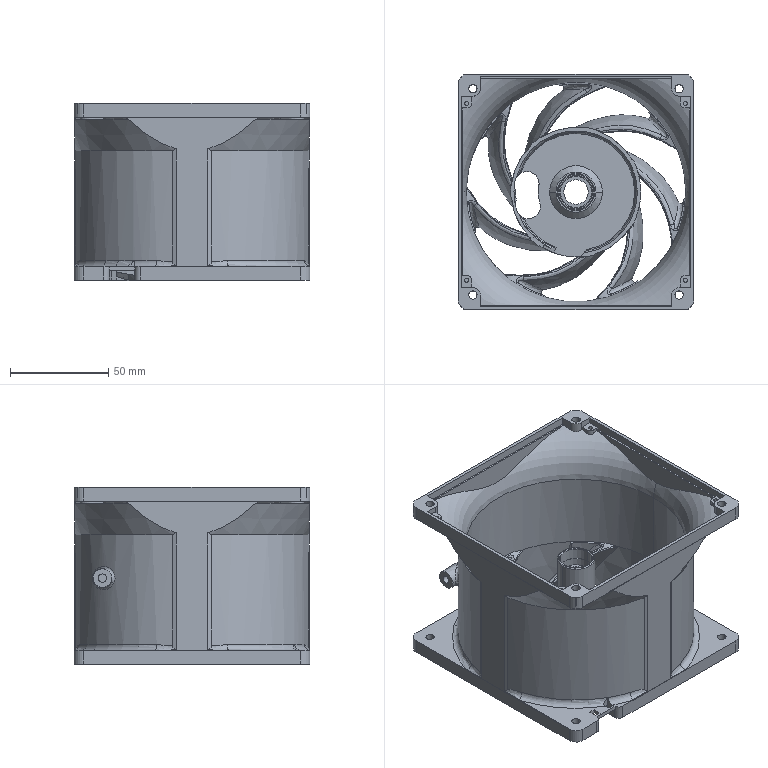NC program | NX | posted with a generic post | part box 120 x 120 x 90.2 mm
Lines 95260 to 96379 of 828686:
(等高精加工_COPY_COPY_COPY , TOOL : 4R0.5)
N190506 T08 M6
N190508 G54
N190510 G17 G0 G90 X-54.5 Y-42.233 S8000 M3
N190512 G43 Z140.7 H8
N190514 Z91.14
N190516 G94 G1 Z90.14 F1500.
N190518 X-54.89 Y-42.272
N190520 X-55.265 Y-42.386
N190522 X-55.611 Y-42.57
N190524 X-55.914 Y-42.819
N190526 X-56.163 Y-43.122
N190528 X-56.348 Y-43.468
N190530 X-56.462 Y-43.843
N190532 X-56.5 Y-44.233
N190534 Y-46.7
N190536 X-54.033
N190538 X-53.896 Z90.126
N190540 X-53.758 Z90.112
N190542 X-53.621 Z90.098
N190544 X-53.484 Z90.084
N190546 X-53.346 Z90.07
N190548 X-56.5
N190550 Y-43.547
N190552 Z90.
N190554 Y-46.7
N190556 X-53.346
N190558 Z89.93
N190560 X-56.5
N190562 Y-43.547
N190564 Z89.86
N190566 Y-46.7
N190568 X-53.346
N190570 Z89.79
N190572 X-56.5
N190574 Y-43.547
N190576 Z89.72
N190578 Y-46.7
N190580 X-53.346
N190582 X-53.347 Z89.65
N190584 X-56.5
N190586 Y-43.547
N190588 Z89.58
N190590 Y-46.7
N190592 X-53.347
N190594 Z89.51
N190596 X-56.5
N190598 Y-43.547
N190600 Z89.44
N190602 Y-46.7
N190604 X-53.347
N190606 Z89.37
N190608 X-56.5
N190610 Y-43.547
N190612 Z89.3
N190614 Y-46.7
N190616 X-53.347
N190618 Z89.23
N190620 X-56.5
N190622 Y-43.547
N190624 Z89.16
N190626 Y-46.7
N190628 X-53.347
N190630 Z89.09
N190632 X-56.5
N190634 Y-43.547
N190636 Z89.02
N190638 Y-46.7
N190640 X-53.347
N190642 Z88.95
N190644 X-56.5
N190646 Y-43.547
N190648 Z88.88
N190650 Y-46.7
N190652 X-53.347
N190654 Z88.81
N190656 X-56.5
N190658 Y-43.547
N190660 Z88.74
N190662 Y-46.7
N190664 X-53.347
N190666 Z88.67
N190668 X-56.5
N190670 Y-43.547
N190672 Z88.6
N190674 Y-46.7
N190676 X-53.347
N190678 Z88.53
N190680 X-56.5
N190682 Y-43.547
N190684 Z88.46
N190686 Y-46.7
N190688 X-53.347
N190690 Z88.39
N190692 X-56.5
N190694 Y-43.547
N190696 Z88.32
N190698 Y-46.7
N190700 X-53.347
N190702 Z88.25
N190704 X-56.5
N190706 Y-43.547
N190708 Z88.18
N190710 Y-46.7
N190712 X-53.347
N190714 Z88.11
N190716 X-56.5
N190718 Y-43.547
N190720 Z88.04
N190722 Y-46.7
N190724 X-53.347
N190726 Z87.97
N190728 X-56.5
N190730 Y-43.547
N190732 Z87.9
N190734 Y-46.7
N190736 X-53.347
N190738 Z87.83
N190740 X-56.5
N190742 Y-43.547
N190744 Z87.76
N190746 Y-46.7
N190748 X-53.347
N190750 Z87.69
N190752 X-56.5
N190754 Y-43.547
N190756 Z87.62
N190758 Y-46.7
N190760 X-53.347
N190762 Z87.55
N190764 X-56.5
N190766 Y-43.547
N190768 Z87.48
N190770 Y-46.7
N190772 X-53.347
N190774 Z87.41
N190776 X-56.5
N190778 Y-43.547
N190780 Z87.34
N190782 Y-46.7
N190784 X-53.347
N190786 Z87.27
N190788 X-56.5
N190790 Y-43.547
N190792 Z87.2
N190794 Y-46.7
N190796 X-53.347
N190798 Z87.185
N190800 X-56.5
N190802 Y-43.547
N190804 Z87.161
N190806 Y-46.7
N190808 X-53.347
N190810 Z87.128
N190812 X-56.5
N190814 Y-43.547
N190816 Z87.087
N190818 Y-46.7
N190820 X-53.347
N190822 Z87.038
N190824 X-56.5
N190826 Y-43.547
N190828 Z86.982
N190830 Y-46.7
N190832 X-53.347
N190834 Z86.922
N190836 X-56.5
N190838 Y-43.547
N190840 Z86.857
N190842 Y-46.7
N190844 X-53.347
N190846 Z86.789
N190848 X-56.5
N190850 Y-43.547
N190852 Z86.719
N190854 Y-46.7
N190856 X-53.347
N190858 Z86.649
N190860 X-56.5
N190862 Y-43.547
N190864 Z86.579
N190866 Y-46.7
N190868 X-53.347
N190870 Z86.509
N190872 X-56.5
N190874 Y-43.547
N190876 Z86.439
N190878 Y-46.7
N190880 X-53.347
N190882 Z86.379
N190884 X-56.5
N190886 Y-43.547
N190888 X-56.462 Y-43.157
N190890 X-56.348 Y-42.782
N190892 X-56.163 Y-42.436
N190894 X-55.914 Y-42.133
N190896 X-55.611 Y-41.884
N190898 X-55.265 Y-41.699
N190900 X-54.89 Y-41.585
N190902 X-54.5 Y-41.547
N190904 Z87.379
N190906 G0 Z140.7
N190908 X-44.7 Y-52.032
N190910 Z91.14
N190912 G1 Z90.14
N190914 X-45.09 Y-52.071
N190916 X-45.466 Y-52.185
N190918 X-45.811 Y-52.369
N190920 X-46.114 Y-52.618
N190922 X-46.363 Y-52.921
N190924 X-46.548 Y-53.267
N190926 X-46.662 Y-53.642
N190928 X-46.7 Y-54.032
N190930 Y-56.5
N190932 X-44.232
N190934 X-44.095 Z90.126
N190936 X-43.957 Z90.112
N190938 X-43.819 Z90.098
N190940 X-43.682 Z90.084
N190942 X-43.544 Z90.07
N190944 X-46.7
N190946 Y-53.345
N190948 Z90.
N190950 Y-56.5
N190952 X-43.544
N190954 Z89.93
N190956 X-46.7
N190958 Y-53.345
N190960 Z89.86
N190962 Y-56.5
N190964 X-43.544
N190966 Z89.79
N190968 X-46.7
N190970 Y-53.345
N190972 Y-53.344 Z89.72
N190974 Y-56.5
N190976 X-43.544
N190978 X-43.546 Z89.65
N190980 X-46.7
N190982 Y-53.346
N190984 Y-53.347 Z89.58
N190986 Y-56.5
N190988 X-43.547
N190990 Z89.51
N190992 X-46.7
N190994 Y-53.347
N190996 Z89.44
N190998 Y-56.5
N191000 X-43.547
N191002 Z89.37
N191004 X-46.7
N191006 Y-53.347
N191008 Z89.3
N191010 Y-56.5
N191012 X-43.547
N191014 Z89.23
N191016 X-46.7
N191018 Y-53.347
N191020 Z89.16
N191022 Y-56.5
N191024 X-43.547
N191026 Z89.09
N191028 X-46.7
N191030 Y-53.347
N191032 Z89.02
N191034 Y-56.5
N191036 X-43.547
N191038 Z88.95
N191040 X-46.7
N191042 Y-53.347
N191044 Z88.88
N191046 Y-56.5
N191048 X-43.547
N191050 Z88.81
N191052 X-46.7
N191054 Y-53.347
N191056 Z88.74
N191058 Y-56.5
N191060 X-43.547
N191062 Z88.67
N191064 X-46.7
N191066 Y-53.347
N191068 Z88.6
N191070 Y-56.5
N191072 X-43.547
N191074 Z88.53
N191076 X-46.7
N191078 Y-53.347
N191080 Z88.46
N191082 Y-56.5
N191084 X-43.547
N191086 Z88.39
N191088 X-46.7
N191090 Y-53.347
N191092 Z88.32
N191094 Y-56.5
N191096 X-43.547
N191098 Z88.25
N191100 X-46.7
N191102 Y-53.347
N191104 Z88.18
N191106 Y-56.5
N191108 X-43.547
N191110 Z88.11
N191112 X-46.7
N191114 Y-53.347
N191116 Z88.04
N191118 Y-56.5
N191120 X-43.547
N191122 Z87.97
N191124 X-46.7
N191126 Y-53.347
N191128 Z87.9
N191130 Y-56.5
N191132 X-43.547
N191134 Z87.83
N191136 X-46.7
N191138 Y-53.347
N191140 Z87.76
N191142 Y-56.5
N191144 X-43.547
N191146 Z87.69
N191148 X-46.7
N191150 Y-53.347
N191152 Z87.62
N191154 Y-56.5
N191156 X-43.547
N191158 Z87.55
N191160 X-46.7
N191162 Y-53.347
N191164 Z87.48
N191166 Y-56.5
N191168 X-43.547
N191170 Z87.41
N191172 X-46.7
N191174 Y-53.347
N191176 Z87.34
N191178 Y-56.5
N191180 X-43.547
N191182 Z87.27
N191184 X-46.7
N191186 Y-53.347
N191188 Z87.2
N191190 Y-56.5
N191192 X-43.547
N191194 X-43.157 Y-56.462
N191196 X-42.782 Y-56.348
N191198 X-42.436 Y-56.163
N191200 X-42.133 Y-55.914
N191202 X-41.884 Y-55.611
N191204 X-41.699 Y-55.265
N191206 X-41.585 Y-54.89
N191208 X-41.547 Y-54.5
N191210 Z88.2
N191212 G0 Z93.7
N191214 X-36.235
N191216 Z88.185
N191218 G1 Z87.185
N191220 X-36.273 Y-54.89
N191222 X-36.387 Y-55.265
N191224 X-36.572 Y-55.611
N191226 X-36.821 Y-55.914
N191228 X-37.124 Y-56.163
N191230 X-37.47 Y-56.348
N191232 X-37.845 Y-56.462
N191234 X-38.235 Y-56.5
N191236 X-41.078
N191238 Y-55.5
N191240 X-41.102 Y-55.061
N191242 X-41.172 Y-54.628
N191244 X-41.115 Y-54.701 Z87.173
N191246 X-41.069 Y-54.776 Z87.161
N191248 X-41.022 Y-55.137
N191250 X-41.006 Y-55.5
N191252 Y-56.5
N191254 X-38.235
N191256 Z87.128
N191258 X-40.941
N191260 Y-55.5
N191262 X-40.973 Y-54.982
N191264 X-41.067 Y-54.471
N191266 X-40.986 Y-54.562 Z87.087
N191268 X-40.909 Y-55.028
N191270 X-40.883 Y-55.5
N191272 Y-56.5
N191274 X-38.056
N191276 X-37.967 Z87.038
N191278 X-40.831
N191280 Y-55.5
N191282 X-40.854 Y-55.059
N191284 X-40.92 Y-54.623
N191286 X-41.03 Y-54.196
N191288 X-40.981 Y-54.279 Z87.01
N191290 X-40.936 Y-54.365 Z86.982
N191292 X-40.825 Y-54.927
N191294 X-40.787 Y-55.5
N191296 Y-56.5
N191298 X-37.967
N191300 X-37.908 Z86.922
N191302 X-40.752
N191304 Y-55.5
N191306 X-40.786 Y-54.95
N191308 X-40.888 Y-54.408
N191310 X-40.853 Y-54.438 Z86.857
N191312 X-40.757 Y-54.965
N191314 X-40.725 Y-55.5
N191316 Y-56.5
N191318 X-37.867
N191320 X-37.839 Z86.789
N191322 X-40.708
N191324 Y-55.5
N191326 X-40.731 Y-55.045
N191328 X-40.8 Y-54.594
N191330 X-40.792 Y-54.598 Z86.719
N191332 X-40.723 Y-55.047
N191334 X-40.7 Y-55.5
N191336 Y-56.5
N191338 X-37.824
N191340 X-37.819 Z86.649
N191342 X-40.7
N191344 Y-55.5
N191346 X-40.726 Y-55.019
N191348 X-40.803 Y-54.543
N191350 X-40.93 Y-54.079
N191352 Z86.579
N191354 X-40.803 Y-54.543
N191356 X-40.726 Y-55.019
N191358 X-40.7 Y-55.5
N191360 Y-56.5
N191362 X-37.819
N191364 Z86.509
N191366 X-40.7
N191368 Y-55.5
N191370 X-40.726 Y-55.019
N191372 X-40.803 Y-54.543
N191374 X-40.93 Y-54.079
N191376 Z86.439
N191378 X-40.803 Y-54.543
N191380 X-40.726 Y-55.019
N191382 X-40.7 Y-55.5
N191384 Y-56.5
N191386 X-37.819
N191388 Z86.379
N191390 X-40.7
N191392 Y-55.5
N191394 X-40.726 Y-55.019
N191396 X-40.803 Y-54.543
N191398 X-40.93 Y-54.079
N191400 X-41.017 Y-53.696
N191402 X-41.028 Y-53.304
N191404 X-40.962 Y-52.918
N191406 X-40.821 Y-52.552
N191408 X-40.612 Y-52.22
N191410 X-40.343 Y-51.935
N191412 X-40.023 Y-51.709
N191414 X-39.664 Y-51.549
N191416 Z87.379
N191418 G0 Z140.7
N191420 X-46.824 Y-46.914
N191422 Z88.185
N191424 G1 Z87.185
N191426 X-47.141 Y-47.146
N191428 X-47.406 Y-47.434
N191430 X-47.61 Y-47.769
N191432 X-47.745 Y-48.137
N191434 X-47.805 Y-48.525
N191436 X-47.789 Y-48.916
N191438 X-47.696 Y-49.297
N191440 X-47.531 Y-49.653
N191442 X-47.244 Y-50.203
N191444 X-47.015 Y-50.781
N191446 X-46.847 Y-51.378
N191448 X-45.519
N191450 X-45.628 Y-51.338 Z87.173
N191452 X-45.736 Y-51.306 Z87.161
N191454 X-46.864
N191456 X-47.031 Y-50.734
N191458 X-47.254 Y-50.181
N191460 X-47.531 Y-49.653
N191462 Z87.128
N191464 X-47.264 Y-50.161
N191466 X-47.046 Y-50.692
N191468 X-46.88 Y-51.241
N191470 X-45.342
N191472 X-45.41 Y-51.21 Z87.107
N191474 X-45.478 Y-51.183 Z87.087
N191476 X-46.895
N191478 X-47.075 Y-50.612
N191480 X-47.311 Y-50.061
N191482 X-47.601 Y-49.537
N191484 X-47.637 Y-49.48 Z87.038
N191486 X-47.339 Y-50.005
N191488 X-47.096 Y-50.557
N191490 X-46.909 Y-51.131
N191492 X-45.2
N191494 X-45.101 Y-51.132
N191496 X-45.002 Y-51.136
N191498 X-45.121 Y-51.108 Z87.01
N191500 X-45.24 Y-51.087 Z86.982
N191502 X-46.921
N191504 X-47.107 Y-50.529
N191506 X-47.346 Y-49.992
N191508 X-47.637 Y-49.48
N191510 X-47.662 Y-49.442 Z86.922
N191512 X-47.365 Y-49.954
N191514 X-47.121 Y-50.492
N191516 X-46.931 Y-51.052
N191518 X-45.308
N191520 X-45.353 Y-51.025 Z86.857
N191522 X-46.938
N191524 X-47.132 Y-50.465
N191526 X-47.379 Y-49.927
N191528 X-47.679 Y-49.416
N191530 X-47.69 Y-49.398 Z86.789
N191532 X-47.388 Y-49.909
N191534 X-47.139 Y-50.448
N191536 X-46.944 Y-51.008
N191538 X-45.563
N191540 X-45.57 Y-51. Z86.719
N191542 X-46.946
N191544 X-47.142 Y-50.439
N191546 X-47.393 Y-49.9
N191548 X-47.697 Y-49.388
N191550 X-47.699 Y-49.385 Z86.649
N191552 X-47.395 Y-49.898
N191554 X-47.143 Y-50.438
N191556 X-46.946 Y-51.
N191558 X-45.2
N191560 X-45.044 Y-51.003
N191562 X-44.888 Y-51.011
N191564 Z86.579
N191566 X-45.044 Y-51.003
N191568 X-45.2 Y-51.
N191570 X-46.946
N191572 X-47.143 Y-50.438
N191574 X-47.395 Y-49.898
N191576 X-47.699 Y-49.385
N191578 Z86.509
N191580 X-47.395 Y-49.898
N191582 X-47.143 Y-50.438
N191584 X-46.946 Y-51.
N191586 X-45.2
N191588 X-45.044 Y-51.003
N191590 X-44.888 Y-51.011
N191592 Z86.439
N191594 X-45.044 Y-51.003
N191596 X-45.2 Y-51.
N191598 X-46.946
N191600 X-47.143 Y-50.438
N191602 X-47.395 Y-49.898
N191604 X-47.699 Y-49.385
N191606 Z86.379
N191608 X-47.395 Y-49.898
N191610 X-47.143 Y-50.438
N191612 X-46.946 Y-51.
N191614 X-45.2
N191616 X-45.044 Y-51.003
N191618 X-44.888 Y-51.011
N191620 Z86.32
N191622 X-45.044 Y-51.003
N191624 X-45.2 Y-51.
N191626 X-46.946
N191628 X-47.143 Y-50.438
N191630 X-47.395 Y-49.898
N191632 X-47.699 Y-49.385
N191634 Z86.26
N191636 X-47.395 Y-49.898
N191638 X-47.143 Y-50.438
N191640 X-46.946 Y-51.
N191642 X-45.2
N191644 X-45.044 Y-51.003
N191646 X-44.888 Y-51.011
N191648 Z86.2
N191650 X-45.044 Y-51.003
N191652 X-45.2 Y-51.
N191654 X-46.946
N191656 X-47.143 Y-50.438
N191658 X-47.395 Y-49.898
N191660 X-47.699 Y-49.385
N191662 Z86.185
N191664 X-47.395 Y-49.898
N191666 X-47.143 Y-50.438
N191668 X-46.946 Y-51.
N191670 X-45.2
N191672 X-45.044 Y-51.003
N191674 X-44.888 Y-51.011
N191676 Z86.161
N191678 X-45.044 Y-51.003
N191680 X-45.2 Y-51.
N191682 X-46.946
N191684 X-47.143 Y-50.438
N191686 X-47.395 Y-49.898
N191688 X-47.699 Y-49.385
N191690 Z86.128
N191692 X-47.395 Y-49.898
N191694 X-47.143 Y-50.438
N191696 X-46.946 Y-51.
N191698 X-45.2
N191700 X-45.044 Y-51.003
N191702 X-44.888 Y-51.011
N191704 Z86.087
N191706 X-45.044 Y-51.003
N191708 X-45.2 Y-51.
N191710 X-46.946
N191712 X-47.143 Y-50.438
N191714 X-47.395 Y-49.898
N191716 X-47.699 Y-49.385
N191718 Z86.038
N191720 X-47.395 Y-49.898
N191722 X-47.143 Y-50.438
N191724 X-46.946 Y-51.
N191726 X-45.2
N191728 X-45.044 Y-51.003
N191730 X-44.888 Y-51.011
N191732 Z85.983
N191734 X-45.044 Y-51.003
N191736 X-45.2 Y-51.
N191738 X-46.946
N191740 X-47.143 Y-50.438
N191742 X-47.395 Y-49.898
N191744 X-47.699 Y-49.385
N191746 Z85.976
N191748 X-47.395 Y-49.898
N191750 X-47.143 Y-50.438
N191752 X-46.946 Y-51.
N191754 X-45.2
N191756 X-45.044 Y-51.003
N191758 X-44.888 Y-51.011
N191760 Z85.969
N191762 X-45.044 Y-51.003
N191764 X-45.2 Y-51.
N191766 X-46.946
N191768 X-47.143 Y-50.438
N191770 X-47.395 Y-49.898
N191772 X-47.699 Y-49.385
N191774 Z85.963
N191776 X-47.395 Y-49.898
N191778 X-47.143 Y-50.438
N191780 X-46.946 Y-51.
N191782 X-45.2
N191784 X-45.044 Y-51.003
N191786 X-44.888 Y-51.011
N191788 Z85.956
N191790 X-45.044 Y-51.003
N191792 X-45.2 Y-51.
N191794 X-46.946
N191796 X-47.143 Y-50.438
N191798 X-47.395 Y-49.898
N191800 X-47.699 Y-49.385
N191802 Z85.949
N191804 X-47.395 Y-49.898
N191806 X-47.143 Y-50.438
N191808 X-46.946 Y-51.
N191810 X-45.2
N191812 X-45.044 Y-51.003
N191814 X-44.888 Y-51.011
N191816 Z85.942
N191818 X-45.044 Y-51.003
N191820 X-45.2 Y-51.
N191822 X-46.946
N191824 X-47.143 Y-50.438
N191826 X-47.395 Y-49.898
N191828 X-47.699 Y-49.385
N191830 Z85.935
N191832 X-47.395 Y-49.898
N191834 X-47.143 Y-50.438
N191836 X-46.946 Y-51.
N191838 X-45.2
N191840 X-45.044 Y-51.003
N191842 X-44.888 Y-51.011
N191844 Z85.927
N191846 X-45.044 Y-51.003
N191848 X-45.2 Y-51.
N191850 X-46.946
N191852 X-47.143 Y-50.438
N191854 X-47.395 Y-49.898
N191856 X-47.699 Y-49.385
N191858 Z85.919
N191860 X-47.395 Y-49.898
N191862 X-47.143 Y-50.438
N191864 X-46.946 Y-51.
N191866 X-45.2
N191868 X-45.044 Y-51.003
N191870 X-44.888 Y-51.011
N191872 Z85.911
N191874 X-45.044 Y-51.003
N191876 X-45.2 Y-51.
N191878 X-46.946
N191880 X-47.143 Y-50.438
N191882 X-47.395 Y-49.898
N191884 X-47.699 Y-49.385
N191886 Z85.903
N191888 X-47.395 Y-49.898
N191890 X-47.143 Y-50.438
N191892 X-46.946 Y-51.
N191894 X-45.2
N191896 X-45.044 Y-51.003
N191898 X-44.888 Y-51.011
N191900 Z85.894
N191902 X-45.044 Y-51.003
N191904 X-45.2 Y-51.
N191906 X-46.946
N191908 X-47.143 Y-50.438
N191910 X-47.395 Y-49.898
N191912 X-47.699 Y-49.385
N191914 Z85.886
N191916 X-47.395 Y-49.898
N191918 X-47.143 Y-50.438
N191920 X-46.946 Y-51.
N191922 X-45.2
N191924 X-45.044 Y-51.003
N191926 X-44.888 Y-51.011
N191928 Z85.877
N191930 X-45.044 Y-51.003
N191932 X-45.2 Y-51.
N191934 X-46.946
N191936 X-47.143 Y-50.438
N191938 X-47.395 Y-49.898
N191940 X-47.699 Y-49.385
N191942 Z85.867
N191944 X-47.395 Y-49.898
N191946 X-47.143 Y-50.438
N191948 X-46.946 Y-51.
N191950 X-45.2
N191952 X-45.044 Y-51.003
N191954 X-44.888 Y-51.011
N191956 Z85.858
N191958 X-45.044 Y-51.003
N191960 X-45.2 Y-51.
N191962 X-46.946
N191964 X-47.143 Y-50.438
N191966 X-47.395 Y-49.898
N191968 X-47.699 Y-49.385
N191970 Z85.848
N191972 X-47.395 Y-49.898
N191974 X-47.143 Y-50.438
N191976 X-46.946 Y-51.
N191978 X-45.2
N191980 X-45.044 Y-51.003
N191982 X-44.888 Y-51.011
N191984 Z85.838
N191986 X-45.044 Y-51.003
N191988 X-45.2 Y-51.
N191990 X-46.946
N191992 X-47.143 Y-50.438
N191994 X-47.395 Y-49.898
N191996 X-47.699 Y-49.385
N191998 Z85.828
N192000 X-47.395 Y-49.898
N192002 X-47.143 Y-50.438
N192004 X-46.946 Y-51.
N192006 X-45.2
N192008 X-45.044 Y-51.003
N192010 X-44.888 Y-51.011
N192012 Z85.817
N192014 X-45.044 Y-51.003
N192016 X-45.2 Y-51.
N192018 X-46.946
N192020 X-47.143 Y-50.438
N192022 X-47.395 Y-49.898
N192024 X-47.699 Y-49.385
N192026 Z85.807
N192028 X-47.395 Y-49.898
N192030 X-47.143 Y-50.438
N192032 X-46.946 Y-51.
N192034 X-45.2
N192036 X-45.044 Y-51.003
N192038 X-44.888 Y-51.011
N192040 Z85.796
N192042 X-45.044 Y-51.003
N192044 X-45.2 Y-51.
N192046 X-46.946
N192048 X-47.143 Y-50.438
N192050 X-47.395 Y-49.898
N192052 X-47.699 Y-49.385
N192054 Z85.785
N192056 X-47.395 Y-49.898
N192058 X-47.143 Y-50.438
N192060 X-46.946 Y-51.
N192062 X-45.2
N192064 X-45.044 Y-51.003
N192066 X-44.888 Y-51.011
N192068 Z85.773
N192070 X-45.044 Y-51.003
N192072 X-45.2 Y-51.
N192074 X-46.946
N192076 X-47.143 Y-50.438
N192078 X-47.395 Y-49.898
N192080 X-47.699 Y-49.385
N192082 Z85.761
N192084 X-47.395 Y-49.898
N192086 X-47.143 Y-50.438
N192088 X-46.946 Y-51.
N192090 X-45.2
N192092 X-45.044 Y-51.003
N192094 X-44.888 Y-51.011
N192096 Z85.75
N192098 X-45.044 Y-51.003
N192100 X-45.2 Y-51.
N192102 X-46.946
N192104 X-47.143 Y-50.438
N192106 X-47.395 Y-49.898
N192108 X-47.699 Y-49.385
N192110 Z85.737
N192112 X-47.395 Y-49.898
N192114 X-47.143 Y-50.438
N192116 X-46.946 Y-51.
N192118 X-45.2
N192120 X-45.044 Y-51.003
N192122 X-44.888 Y-51.011
N192124 Z85.725
N192126 X-45.044 Y-51.003
N192128 X-45.2 Y-51.
N192130 X-46.946
N192132 X-47.143 Y-50.438
N192134 X-47.395 Y-49.898
N192136 X-47.699 Y-49.385
N192138 Z85.713
N192140 X-47.395 Y-49.898
N192142 X-47.143 Y-50.438
N192144 X-46.946 Y-51.
N192146 X-45.2
N192148 X-45.044 Y-51.003
N192150 X-44.888 Y-51.011
N192152 Z85.7
N192154 X-45.044 Y-51.003
N192156 X-45.2 Y-51.
N192158 X-46.946
N192160 X-47.143 Y-50.438
N192162 X-47.395 Y-49.898
N192164 X-47.699 Y-49.385
N192166 Z85.687
N192168 X-47.395 Y-49.898
N192170 X-47.143 Y-50.438
N192172 X-46.946 Y-51.
N192174 X-45.2
N192176 X-45.044 Y-51.003
N192178 X-44.888 Y-51.011
N192180 Z85.673
N192182 X-45.044 Y-51.003
N192184 X-45.2 Y-51.
N192186 X-46.946
N192188 X-47.143 Y-50.438
N192190 X-47.395 Y-49.898
N192192 X-47.699 Y-49.385
N192194 Z85.66
N192196 X-47.395 Y-49.898
N192198 X-47.143 Y-50.438
N192200 X-46.946 Y-51.
N192202 X-45.2
N192204 X-45.044 Y-51.003
N192206 X-44.888 Y-51.011
N192208 Z85.646
N192210 X-45.044 Y-51.003
N192212 X-45.2 Y-51.
N192214 X-46.946
N192216 X-47.143 Y-50.438
N192218 X-47.395 Y-49.898
N192220 X-47.699 Y-49.385
N192222 Z85.632
N192224 X-47.395 Y-49.898
N192226 X-47.143 Y-50.438
N192228 X-46.946 Y-51.
N192230 X-45.2
N192232 X-45.044 Y-51.003
N192234 X-44.888 Y-51.011
N192236 Z85.618
N192238 X-45.044 Y-51.003
N192240 X-45.2 Y-51.
N192242 X-46.946
N192244 X-47.143 Y-50.438
N192246 X-47.395 Y-49.898
N192248 X-47.699 Y-49.385
N192250 Z85.603
N192252 X-47.395 Y-49.898
N192254 X-47.143 Y-50.438
N192256 X-46.946 Y-51.
N192258 X-45.2
N192260 X-45.044 Y-51.003
N192262 X-44.888 Y-51.011
N192264 Z85.589
N192266 X-45.044 Y-51.003
N192268 X-45.2 Y-51.
N192270 X-46.946
N192272 X-47.143 Y-50.438
N192274 X-47.395 Y-49.898
N192276 X-47.699 Y-49.385
N192278 Z85.574
N192280 X-47.395 Y-49.898
N192282 X-47.143 Y-50.438
N192284 X-46.946 Y-51.
N192286 X-45.2
N192288 X-45.044 Y-51.003
N192290 X-44.888 Y-51.011
N192292 Z85.559
N192294 X-45.044 Y-51.003
N192296 X-45.2 Y-51.
N192298 X-46.946
N192300 X-47.143 Y-50.438
N192302 X-47.395 Y-49.898
N192304 X-47.699 Y-49.385
N192306 Z85.543
N192308 X-47.395 Y-49.898
N192310 X-47.143 Y-50.438
N192312 X-46.946 Y-51.
N192314 X-45.2
N192316 X-45.044 Y-51.003
N192318 X-44.888 Y-51.011
N192320 Z85.528
N192322 X-45.044 Y-51.003
N192324 X-45.2 Y-51.
N192326 X-46.946
N192328 X-47.143 Y-50.438
N192330 X-47.395 Y-49.898
N192332 X-47.699 Y-49.385
N192334 Z85.512
N192336 X-47.395 Y-49.898
N192338 X-47.143 Y-50.438
N192340 X-46.946 Y-51.
N192342 X-45.2
N192344 X-45.044 Y-51.003
N192346 X-44.888 Y-51.011
N192348 Z85.496
N192350 X-45.044 Y-51.003
N192352 X-45.2 Y-51.
N192354 X-46.946
N192356 X-47.143 Y-50.438
N192358 X-47.395 Y-49.898
N192360 X-47.699 Y-49.385
N192362 X-47.714 Y-49.363 Z85.479
N192364 X-47.403 Y-49.882
N192366 X-47.146 Y-50.429
N192368 X-46.946 Y-51.
N192370 X-45.2
N192372 X-45.044 Y-51.003
N192374 X-44.888 Y-51.011
N192376 X-44.88 Z85.463
N192378 X-45.04 Y-51.003
N192380 X-45.2 Y-51.
N192382 X-46.946
N192384 X-47.159 Y-50.399
N192386 X-47.434 Y-49.824
N192388 X-47.769 Y-49.281
N192390 X-47.699 Y-49.385 Z85.446
N192392 X-47.395 Y-49.898
N192394 X-47.143 Y-50.438
N192396 X-46.946 Y-51.
N192398 X-45.2
N192400 X-45.044 Y-51.003
N192402 X-44.888 Y-51.011
N192404 Z85.429
N192406 X-45.044 Y-51.003
N192408 X-45.2 Y-51.
N192410 X-46.946
N192412 X-47.143 Y-50.438
N192414 X-47.395 Y-49.898
N192416 X-47.699 Y-49.385
N192418 Z85.412
N192420 X-47.395 Y-49.898
N192422 X-47.143 Y-50.438
N192424 X-46.946 Y-51.
N192426 X-45.2
N192428 X-45.044 Y-51.003
N192430 X-44.888 Y-51.011
N192432 X-44.886 Z85.394
N192434 X-45.043 Y-51.003
N192436 X-45.2 Y-51.
N192438 X-46.867
N192440 X-46.922 Y-50.95
N192442 X-46.977 Y-50.899
N192444 X-47.17 Y-50.372
N192446 X-47.412 Y-49.866
N192448 X-47.7 Y-49.384
N192450 X-47.699 Y-49.385 Z85.376
N192452 X-47.434 Y-49.825
N192454 X-47.207 Y-50.287
N192456 X-47.02 Y-50.766
N192458 X-46.893 Y-50.883
N192460 X-46.767 Y-51.
N192462 X-45.2
N192464 X-45.044 Y-51.003
N192466 X-44.887 Y-51.011
N192468 X-44.799 Y-51.018 Z85.359
N192470 X-44.999 Y-51.004
N192472 X-45.2 Y-51.
N192474 X-46.666
N192476 X-46.868 Y-50.815
N192478 X-47.069 Y-50.628
N192480 X-47.257 Y-50.174
N192482 X-47.482 Y-49.738
N192484 X-47.742 Y-49.32
N192486 X-47.735 Y-49.331 Z85.34
N192488 X-47.398 Y-49.891
N192490 X-47.124 Y-50.484
N192492 X-46.845 Y-50.743
N192494 X-46.565 Y-51.
N192496 X-45.2
N192498 X-45.006 Y-51.004
N192500 X-44.813 Y-51.017
N192502 X-44.833 Y-51.015 Z85.322
N192504 X-45.016 Y-51.004
N192506 X-45.2 Y-51.
N192508 X-46.465
N192510 X-46.827 Y-50.668
N192512 X-47.187 Y-50.333
N192514 X-47.433 Y-49.827
N192516 X-47.725 Y-49.346
N192518 X-47.778 Y-49.269 Z85.303
N192520 X-47.498 Y-49.709
N192522 X-47.258 Y-50.173
N192524 X-46.813 Y-50.588
N192526 X-46.364 Y-51.
N192528 X-45.2
N192530 X-44.965 Y-51.006
N192532 X-44.731 Y-51.025
N192534 X-44.773 Y-51.02 Z85.284
N192536 X-44.986 Y-51.005
N192538 X-45.2 Y-51.
N192540 X-46.264
N192542 X-46.805 Y-50.504
N192544 X-47.341 Y-50.001
N192546 X-47.537 Y-49.644
N192548 X-47.756 Y-49.301
N192550 X-47.81 Y-49.223 Z85.278
N192552 X-47.866 Y-49.146 Z85.272
N192554 X-47.923 Y-49.069 Z85.265
N192556 X-47.667 Y-49.433
N192558 X-47.439 Y-49.815
N192560 X-46.805 Y-50.412
N192562 X-46.163 Y-51.
N192564 X-45.2
N192566 X-45.03 Y-51.003
N192568 X-44.861 Y-51.013
N192570 X-44.786 Y-51.019 Z85.246
N192572 X-44.993 Y-51.005
N192574 X-45.2 Y-51.
N192576 X-46.062
N192578 X-46.554 Y-50.552
N192580 X-47.041 Y-50.099
N192582 X-46.934 Y-50.106 Z85.226
N192584 X-46.45 Y-50.556
N192586 X-45.962 Y-51.
N192588 X-45.2
N192590 X-44.959 Y-51.006
N192592 X-44.719 Y-51.026
N192594 X-44.627 Y-51.037 Z85.207
N192596 X-44.913 Y-51.009
N192598 X-45.2 Y-51.
N192600 X-45.861
N192602 X-46.339 Y-50.566
N192604 X-46.813 Y-50.128
N192606 X-46.715 Y-50.127 Z85.187
N192608 X-46.24 Y-50.566
N192610 X-45.76 Y-51.
N192612 X-45.2
N192614 X-44.895 Y-51.01
N192616 X-44.591 Y-51.041
N192618 X-44.492 Y-51.056 Z85.166
N192620 X-44.845 Y-51.014
N192622 X-45.2 Y-51.
N192624 X-45.66
N192626 X-46.127 Y-50.577
N192628 X-46.591 Y-50.15
N192630 X-46.487 Y-50.155 Z85.146
N192632 X-46.025 Y-50.58
N192634 X-45.559 Y-51.
N192636 X-45.2
N192638 X-44.828 Y-51.015
N192640 X-44.458 Y-51.062
N192642 X-44.36 Y-51.079 Z85.125
N192644 X-44.778 Y-51.02
N192646 X-45.2 Y-51.
N192648 X-45.458
N192650 X-45.912 Y-50.592
N192652 X-46.362 Y-50.18
N192654 X-46.251 Y-50.191 Z85.104
N192656 X-45.806 Y-50.597
N192658 X-45.357 Y-51.
N192660 X-45.2
N192662 X-44.717 Y-51.026
N192664 X-44.241 Y-51.103
N192666 X-44.228 Y-51.106 Z85.083
N192668 X-44.711 Y-51.027
N192670 X-45.2 Y-51.
N192672 X-45.257
N192674 X-45.692 Y-50.611
N192676 X-46.123 Y-50.218
N192678 X-46.005 Y-50.236 Z85.062
N192680 X-45.582 Y-50.62
N192682 X-45.156 Y-51.
N192684 X-44.632 Y-51.036
N192686 X-44.116 Y-51.132
N192688 X-44.031 Y-51.154 Z85.051
N192690 X-43.946 Y-51.178 Z85.04
N192692 X-44.494 Y-51.056
N192694 X-45.052 Y-51.002
N192696 X-45.464 Y-50.636
N192698 X-45.872 Y-50.266
N192700 X-45.745 Y-50.292 Z85.018
N192702 X-45.347 Y-50.651
N192704 X-44.946 Y-51.007
N192706 X-44.483 Y-51.057
N192708 X-44.028 Y-51.155
N192710 X-43.95 Y-51.177 Z84.996
N192712 X-44.389 Y-51.074
N192714 X-44.837 Y-51.015
N192716 X-45.223 Y-50.673
N192718 X-45.607 Y-50.328
N192720 X-45.537 Y-50.346 Z84.985
N192722 X-45.468 Y-50.364 Z84.974
N192724 X-45.097 Y-50.696
N192726 X-44.724 Y-51.025
N192728 X-44.292 Y-51.093
N192730 X-43.869 Y-51.201
N192732 X-43.786 Y-51.228 Z84.951
N192734 X-44.192 Y-51.114
N192736 X-44.607 Y-51.039
N192738 X-44.972 Y-50.718